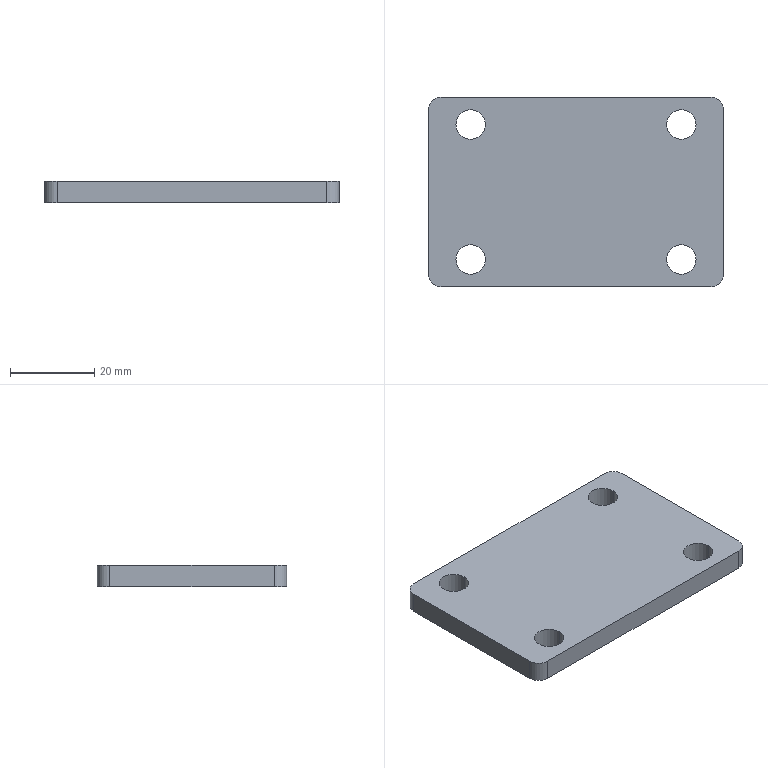Part | SolidWorks | features BaseBody 1 | 1 solid | 18 faces | box 70 x 45 x 5 mm | volume 14942 mm3 | cylinder 12 | plane 6 | commonest cylinder face diameters 7 x8 6 x4
STEP:
#1=CARTESIAN_POINT('',(21.5,-16.,5.));
#2=VERTEX_POINT('',#1);
#3=CARTESIAN_POINT('',(28.5,-16.,5.));
#4=VERTEX_POINT('',#3);
#5=CARTESIAN_POINT('',(25.,-16.,5.));
#6=DIRECTION('',(0.,0.,1.));
#7=DIRECTION('',(1.,0.,0.));
#8=AXIS2_PLACEMENT_3D('',#5,#6,#7);
#9=CIRCLE('',#8,3.5);
#10=EDGE_CURVE('',#2,#4,#9,.T.);
#11=ORIENTED_EDGE('',*,*,#10,.T.);
#12=CARTESIAN_POINT('',(28.5,-16.,0.));
#13=VERTEX_POINT('',#12);
#14=CARTESIAN_POINT('',(28.5,-16.,5.));
#15=DIRECTION('',(0.,0.,-1.));
#16=VECTOR('',#15,1000.);
#17=LINE('',#14,#16);
#18=EDGE_CURVE('',#4,#13,#17,.T.);
#19=ORIENTED_EDGE('',*,*,#18,.T.);
#20=CARTESIAN_POINT('',(21.5,-16.,0.));
#21=VERTEX_POINT('',#20);
#22=CARTESIAN_POINT('',(25.,-16.,0.));
#23=DIRECTION('',(0.,0.,1.));
#24=DIRECTION('',(1.,0.,0.));
#25=AXIS2_PLACEMENT_3D('',#22,#23,#24);
#26=CIRCLE('',#25,3.5);
#27=EDGE_CURVE('',#21,#13,#26,.T.);
#28=ORIENTED_EDGE('',*,*,#27,.F.);
#29=CARTESIAN_POINT('',(21.5,-16.,5.));
#30=DIRECTION('',(0.,0.,-1.));
#31=VECTOR('',#30,1000.);
#32=LINE('',#29,#31);
#33=EDGE_CURVE('',#2,#21,#32,.T.);
#34=ORIENTED_EDGE('',*,*,#33,.F.);
#35=EDGE_LOOP('',(#11,#19,#28,#34));
#36=FACE_OUTER_BOUND('',#35,.T.);
#37=CARTESIAN_POINT('',(25.,-16.,5.));
#38=DIRECTION('',(0.,0.,-1.));
#39=DIRECTION('',(-1.,0.,0.));
#40=AXIS2_PLACEMENT_3D('',#37,#38,#39);
#41=CYLINDRICAL_SURFACE('',#40,3.5);
#42=ADVANCED_FACE('',(#36),#41,.F.);
#43=CARTESIAN_POINT('',(-28.5,-16.,5.));
#44=VERTEX_POINT('',#43);
#45=CARTESIAN_POINT('',(-21.5,-16.,5.));
#46=VERTEX_POINT('',#45);
#47=CARTESIAN_POINT('',(-25.,-16.,5.));
#48=DIRECTION('',(0.,0.,1.));
#49=DIRECTION('',(-1.,0.,0.));
#50=AXIS2_PLACEMENT_3D('',#47,#48,#49);
#51=CIRCLE('',#50,3.5);
#52=EDGE_CURVE('',#44,#46,#51,.T.);
#53=ORIENTED_EDGE('',*,*,#52,.T.);
#54=CARTESIAN_POINT('',(-21.5,-16.,0.));
#55=VERTEX_POINT('',#54);
#56=CARTESIAN_POINT('',(-21.5,-16.,5.));
#57=DIRECTION('',(0.,0.,-1.));
#58=VECTOR('',#57,1000.);
#59=LINE('',#56,#58);
#60=EDGE_CURVE('',#46,#55,#59,.T.);
#61=ORIENTED_EDGE('',*,*,#60,.T.);
#62=CARTESIAN_POINT('',(-28.5,-16.,0.));
#63=VERTEX_POINT('',#62);
#64=CARTESIAN_POINT('',(-25.,-16.,0.));
#65=DIRECTION('',(0.,0.,1.));
#66=DIRECTION('',(-1.,0.,0.));
#67=AXIS2_PLACEMENT_3D('',#64,#65,#66);
#68=CIRCLE('',#67,3.5);
#69=EDGE_CURVE('',#63,#55,#68,.T.);
#70=ORIENTED_EDGE('',*,*,#69,.F.);
#71=CARTESIAN_POINT('',(-28.5,-16.,5.));
#72=DIRECTION('',(0.,0.,-1.));
#73=VECTOR('',#72,1000.);
#74=LINE('',#71,#73);
#75=EDGE_CURVE('',#44,#63,#74,.T.);
#76=ORIENTED_EDGE('',*,*,#75,.F.);
#77=EDGE_LOOP('',(#53,#61,#70,#76));
#78=FACE_OUTER_BOUND('',#77,.T.);
#79=CARTESIAN_POINT('',(-25.,-16.,5.));
#80=DIRECTION('',(0.,0.,-1.));
#81=DIRECTION('',(-1.,0.,0.));
#82=AXIS2_PLACEMENT_3D('',#79,#80,#81);
#83=CYLINDRICAL_SURFACE('',#82,3.5);
#84=ADVANCED_FACE('',(#78),#83,.F.);
#85=CARTESIAN_POINT('',(21.5,16.,5.));
#86=VERTEX_POINT('',#85);
#87=CARTESIAN_POINT('',(28.5,16.,5.));
#88=VERTEX_POINT('',#87);
#89=CARTESIAN_POINT('',(25.,16.,5.));
#90=DIRECTION('',(0.,0.,1.));
#91=DIRECTION('',(-1.,0.,0.));
#92=AXIS2_PLACEMENT_3D('',#89,#90,#91);
#93=CIRCLE('',#92,3.5);
#94=EDGE_CURVE('',#86,#88,#93,.T.);
#95=ORIENTED_EDGE('',*,*,#94,.T.);
#96=CARTESIAN_POINT('',(28.5,16.,0.));
#97=VERTEX_POINT('',#96);
#98=CARTESIAN_POINT('',(28.5,16.,5.));
#99=DIRECTION('',(0.,0.,-1.));
#100=VECTOR('',#99,1000.);
#101=LINE('',#98,#100);
#102=EDGE_CURVE('',#88,#97,#101,.T.);
#103=ORIENTED_EDGE('',*,*,#102,.T.);
#104=CARTESIAN_POINT('',(21.5,16.,0.));
#105=VERTEX_POINT('',#104);
#106=CARTESIAN_POINT('',(25.,16.,0.));
#107=DIRECTION('',(0.,0.,1.));
#108=DIRECTION('',(-1.,0.,0.));
#109=AXIS2_PLACEMENT_3D('',#106,#107,#108);
#110=CIRCLE('',#109,3.5);
#111=EDGE_CURVE('',#105,#97,#110,.T.);
#112=ORIENTED_EDGE('',*,*,#111,.F.);
#113=CARTESIAN_POINT('',(21.5,16.,5.));
#114=DIRECTION('',(0.,0.,-1.));
#115=VECTOR('',#114,1000.);
#116=LINE('',#113,#115);
#117=EDGE_CURVE('',#86,#105,#116,.T.);
#118=ORIENTED_EDGE('',*,*,#117,.F.);
#119=EDGE_LOOP('',(#95,#103,#112,#118));
#120=FACE_OUTER_BOUND('',#119,.T.);
#121=CARTESIAN_POINT('',(25.,16.,5.));
#122=DIRECTION('',(0.,0.,-1.));
#123=DIRECTION('',(-1.,0.,0.));
#124=AXIS2_PLACEMENT_3D('',#121,#122,#123);
#125=CYLINDRICAL_SURFACE('',#124,3.5);
#126=ADVANCED_FACE('',(#120),#125,.F.);
#127=CARTESIAN_POINT('',(-28.5,16.,5.));
#128=VERTEX_POINT('',#127);
#129=CARTESIAN_POINT('',(-21.5,16.,5.));
#130=VERTEX_POINT('',#129);
#131=CARTESIAN_POINT('',(-25.,16.,5.));
#132=DIRECTION('',(0.,0.,1.));
#133=DIRECTION('',(1.,0.,0.));
#134=AXIS2_PLACEMENT_3D('',#131,#132,#133);
#135=CIRCLE('',#134,3.5);
#136=EDGE_CURVE('',#128,#130,#135,.T.);
#137=ORIENTED_EDGE('',*,*,#136,.T.);
#138=CARTESIAN_POINT('',(-21.5,16.,0.));
#139=VERTEX_POINT('',#138);
#140=CARTESIAN_POINT('',(-21.5,16.,5.));
#141=DIRECTION('',(0.,0.,-1.));
#142=VECTOR('',#141,1000.);
#143=LINE('',#140,#142);
#144=EDGE_CURVE('',#130,#139,#143,.T.);
#145=ORIENTED_EDGE('',*,*,#144,.T.);
#146=CARTESIAN_POINT('',(-28.5,16.,0.));
#147=VERTEX_POINT('',#146);
#148=CARTESIAN_POINT('',(-25.,16.,0.));
#149=DIRECTION('',(0.,0.,1.));
#150=DIRECTION('',(1.,0.,0.));
#151=AXIS2_PLACEMENT_3D('',#148,#149,#150);
#152=CIRCLE('',#151,3.5);
#153=EDGE_CURVE('',#147,#139,#152,.T.);
#154=ORIENTED_EDGE('',*,*,#153,.F.);
#155=CARTESIAN_POINT('',(-28.5,16.,5.));
#156=DIRECTION('',(0.,0.,-1.));
#157=VECTOR('',#156,1000.);
#158=LINE('',#155,#157);
#159=EDGE_CURVE('',#128,#147,#158,.T.);
#160=ORIENTED_EDGE('',*,*,#159,.F.);
#161=EDGE_LOOP('',(#137,#145,#154,#160));
#162=FACE_OUTER_BOUND('',#161,.T.);
#163=CARTESIAN_POINT('',(-25.,16.,5.));
#164=DIRECTION('',(0.,0.,-1.));
#165=DIRECTION('',(-1.,0.,0.));
#166=AXIS2_PLACEMENT_3D('',#163,#164,#165);
#167=CYLINDRICAL_SURFACE('',#166,3.5);
#168=ADVANCED_FACE('',(#162),#167,.F.);
#169=CARTESIAN_POINT('',(-35.,19.5,5.));
#170=VERTEX_POINT('',#169);
#171=CARTESIAN_POINT('',(-35.,-19.5,5.));
#172=VERTEX_POINT('',#171);
#173=CARTESIAN_POINT('',(-35.,-22.5,5.));
#174=DIRECTION('',(0.,-1.,0.));
#175=VECTOR('',#174,1000.);
#176=LINE('',#173,#175);
#177=EDGE_CURVE('',#170,#172,#176,.T.);
#178=ORIENTED_EDGE('',*,*,#177,.T.);
#179=CARTESIAN_POINT('',(-32.,-22.5,5.));
#180=VERTEX_POINT('',#179);
#181=CARTESIAN_POINT('',(-32.,-19.5,5.));
#182=DIRECTION('',(0.,0.,1.));
#183=DIRECTION('',(-1.,0.,0.));
#184=AXIS2_PLACEMENT_3D('',#181,#182,#183);
#185=CIRCLE('',#184,3.);
#186=EDGE_CURVE('',#172,#180,#185,.T.);
#187=ORIENTED_EDGE('',*,*,#186,.T.);
#188=CARTESIAN_POINT('',(32.,-22.5,5.));
#189=VERTEX_POINT('',#188);
#190=CARTESIAN_POINT('',(-35.,-22.5,5.));
#191=DIRECTION('',(1.,0.,0.));
#192=VECTOR('',#191,1000.);
#193=LINE('',#190,#192);
#194=EDGE_CURVE('',#180,#189,#193,.T.);
#195=ORIENTED_EDGE('',*,*,#194,.T.);
#196=CARTESIAN_POINT('',(35.,-19.5,5.));
#197=VERTEX_POINT('',#196);
#198=CARTESIAN_POINT('',(32.,-19.5,5.));
#199=DIRECTION('',(0.,0.,1.));
#200=DIRECTION('',(-1.,0.,0.));
#201=AXIS2_PLACEMENT_3D('',#198,#199,#200);
#202=CIRCLE('',#201,3.);
#203=EDGE_CURVE('',#189,#197,#202,.T.);
#204=ORIENTED_EDGE('',*,*,#203,.T.);
#205=CARTESIAN_POINT('',(35.,19.5,5.));
#206=VERTEX_POINT('',#205);
#207=CARTESIAN_POINT('',(35.,-22.5,5.));
#208=DIRECTION('',(0.,1.,0.));
#209=VECTOR('',#208,1000.);
#210=LINE('',#207,#209);
#211=EDGE_CURVE('',#197,#206,#210,.T.);
#212=ORIENTED_EDGE('',*,*,#211,.T.);
#213=CARTESIAN_POINT('',(32.,22.5,5.));
#214=VERTEX_POINT('',#213);
#215=CARTESIAN_POINT('',(32.,19.5,5.));
#216=DIRECTION('',(0.,0.,1.));
#217=DIRECTION('',(-1.,0.,0.));
#218=AXIS2_PLACEMENT_3D('',#215,#216,#217);
#219=CIRCLE('',#218,3.);
#220=EDGE_CURVE('',#206,#214,#219,.T.);
#221=ORIENTED_EDGE('',*,*,#220,.T.);
#222=CARTESIAN_POINT('',(-32.,22.5,5.));
#223=VERTEX_POINT('',#222);
#224=CARTESIAN_POINT('',(-35.,22.5,5.));
#225=DIRECTION('',(-1.,0.,0.));
#226=VECTOR('',#225,1000.);
#227=LINE('',#224,#226);
#228=EDGE_CURVE('',#214,#223,#227,.T.);
#229=ORIENTED_EDGE('',*,*,#228,.T.);
#230=CARTESIAN_POINT('',(-32.,19.5,5.));
#231=DIRECTION('',(0.,0.,1.));
#232=DIRECTION('',(-1.,0.,0.));
#233=AXIS2_PLACEMENT_3D('',#230,#231,#232);
#234=CIRCLE('',#233,3.);
#235=EDGE_CURVE('',#223,#170,#234,.T.);
#236=ORIENTED_EDGE('',*,*,#235,.T.);
#237=EDGE_LOOP('',(#178,#187,#195,#204,#212,#221,#229,#236));
#238=FACE_OUTER_BOUND('',#237,.T.);
#239=ORIENTED_EDGE('',*,*,#136,.F.);
#240=CARTESIAN_POINT('',(-25.,16.,5.));
#241=DIRECTION('',(0.,0.,1.));
#242=DIRECTION('',(1.,0.,0.));
#243=AXIS2_PLACEMENT_3D('',#240,#241,#242);
#244=CIRCLE('',#243,3.5);
#245=EDGE_CURVE('',#130,#128,#244,.T.);
#246=ORIENTED_EDGE('',*,*,#245,.F.);
#247=EDGE_LOOP('',(#239,#246));
#248=FACE_BOUND('',#247,.T.);
#249=ORIENTED_EDGE('',*,*,#94,.F.);
#250=CARTESIAN_POINT('',(25.,16.,5.));
#251=DIRECTION('',(0.,0.,1.));
#252=DIRECTION('',(-1.,0.,0.));
#253=AXIS2_PLACEMENT_3D('',#250,#251,#252);
#254=CIRCLE('',#253,3.5);
#255=EDGE_CURVE('',#88,#86,#254,.T.);
#256=ORIENTED_EDGE('',*,*,#255,.F.);
#257=EDGE_LOOP('',(#249,#256));
#258=FACE_BOUND('',#257,.T.);
#259=ORIENTED_EDGE('',*,*,#52,.F.);
#260=CARTESIAN_POINT('',(-25.,-16.,5.));
#261=DIRECTION('',(0.,0.,1.));
#262=DIRECTION('',(-1.,0.,0.));
#263=AXIS2_PLACEMENT_3D('',#260,#261,#262);
#264=CIRCLE('',#263,3.5);
#265=EDGE_CURVE('',#46,#44,#264,.T.);
#266=ORIENTED_EDGE('',*,*,#265,.F.);
#267=EDGE_LOOP('',(#259,#266));
#268=FACE_BOUND('',#267,.T.);
#269=ORIENTED_EDGE('',*,*,#10,.F.);
#270=CARTESIAN_POINT('',(25.,-16.,5.));
#271=DIRECTION('',(0.,0.,1.));
#272=DIRECTION('',(1.,0.,0.));
#273=AXIS2_PLACEMENT_3D('',#270,#271,#272);
#274=CIRCLE('',#273,3.5);
#275=EDGE_CURVE('',#4,#2,#274,.T.);
#276=ORIENTED_EDGE('',*,*,#275,.F.);
#277=EDGE_LOOP('',(#269,#276));
#278=FACE_BOUND('',#277,.T.);
#279=CARTESIAN_POINT('',(0.,0.,5.));
#280=DIRECTION('',(0.,0.,-1.));
#281=DIRECTION('',(-1.,0.,0.));
#282=AXIS2_PLACEMENT_3D('',#279,#280,#281);
#283=PLANE('',#282);
#284=ADVANCED_FACE('',(#238,#248,#258,#268,#278),#283,.F.);
#285=ORIENTED_EDGE('',*,*,#69,.T.);
#286=CARTESIAN_POINT('',(-25.,-16.,0.));
#287=DIRECTION('',(0.,0.,1.));
#288=DIRECTION('',(-1.,0.,0.));
#289=AXIS2_PLACEMENT_3D('',#286,#287,#288);
#290=CIRCLE('',#289,3.5);
#291=EDGE_CURVE('',#55,#63,#290,.T.);
#292=ORIENTED_EDGE('',*,*,#291,.T.);
#293=EDGE_LOOP('',(#285,#292));
#294=FACE_BOUND('',#293,.T.);
#295=ORIENTED_EDGE('',*,*,#153,.T.);
#296=CARTESIAN_POINT('',(-25.,16.,0.));
#297=DIRECTION('',(0.,0.,1.));
#298=DIRECTION('',(1.,0.,0.));
#299=AXIS2_PLACEMENT_3D('',#296,#297,#298);
#300=CIRCLE('',#299,3.5);
#301=EDGE_CURVE('',#139,#147,#300,.T.);
#302=ORIENTED_EDGE('',*,*,#301,.T.);
#303=EDGE_LOOP('',(#295,#302));
#304=FACE_BOUND('',#303,.T.);
#305=CARTESIAN_POINT('',(-32.,-22.5,0.));
#306=VERTEX_POINT('',#305);
#307=CARTESIAN_POINT('',(32.,-22.5,0.));
#308=VERTEX_POINT('',#307);
#309=CARTESIAN_POINT('',(-35.,-22.5,0.));
#310=DIRECTION('',(1.,0.,0.));
#311=VECTOR('',#310,1000.);
#312=LINE('',#309,#311);
#313=EDGE_CURVE('',#306,#308,#312,.T.);
#314=ORIENTED_EDGE('',*,*,#313,.F.);
#315=CARTESIAN_POINT('',(-35.,-19.5,0.));
#316=VERTEX_POINT('',#315);
#317=CARTESIAN_POINT('',(-32.,-19.5,0.));
#318=DIRECTION('',(0.,0.,-1.));
#319=DIRECTION('',(-1.,0.,0.));
#320=AXIS2_PLACEMENT_3D('',#317,#318,#319);
#321=CIRCLE('',#320,3.);
#322=EDGE_CURVE('',#306,#316,#321,.T.);
#323=ORIENTED_EDGE('',*,*,#322,.T.);
#324=CARTESIAN_POINT('',(-35.,19.5,0.));
#325=VERTEX_POINT('',#324);
#326=CARTESIAN_POINT('',(-35.,-22.5,0.));
#327=DIRECTION('',(0.,-1.,0.));
#328=VECTOR('',#327,1000.);
#329=LINE('',#326,#328);
#330=EDGE_CURVE('',#325,#316,#329,.T.);
#331=ORIENTED_EDGE('',*,*,#330,.F.);
#332=CARTESIAN_POINT('',(-32.,22.5,0.));
#333=VERTEX_POINT('',#332);
#334=CARTESIAN_POINT('',(-32.,19.5,0.));
#335=DIRECTION('',(0.,0.,-1.));
#336=DIRECTION('',(-1.,0.,0.));
#337=AXIS2_PLACEMENT_3D('',#334,#335,#336);
#338=CIRCLE('',#337,3.);
#339=EDGE_CURVE('',#325,#333,#338,.T.);
#340=ORIENTED_EDGE('',*,*,#339,.T.);
#341=CARTESIAN_POINT('',(32.,22.5,0.));
#342=VERTEX_POINT('',#341);
#343=CARTESIAN_POINT('',(-35.,22.5,0.));
#344=DIRECTION('',(-1.,0.,0.));
#345=VECTOR('',#344,1000.);
#346=LINE('',#343,#345);
#347=EDGE_CURVE('',#342,#333,#346,.T.);
#348=ORIENTED_EDGE('',*,*,#347,.F.);
#349=CARTESIAN_POINT('',(35.,19.5,0.));
#350=VERTEX_POINT('',#349);
#351=CARTESIAN_POINT('',(32.,19.5,0.));
#352=DIRECTION('',(0.,0.,-1.));
#353=DIRECTION('',(-1.,0.,0.));
#354=AXIS2_PLACEMENT_3D('',#351,#352,#353);
#355=CIRCLE('',#354,3.);
#356=EDGE_CURVE('',#342,#350,#355,.T.);
#357=ORIENTED_EDGE('',*,*,#356,.T.);
#358=CARTESIAN_POINT('',(35.,-19.5,0.));
#359=VERTEX_POINT('',#358);
#360=CARTESIAN_POINT('',(35.,-22.5,0.));
#361=DIRECTION('',(0.,1.,0.));
#362=VECTOR('',#361,1000.);
#363=LINE('',#360,#362);
#364=EDGE_CURVE('',#359,#350,#363,.T.);
#365=ORIENTED_EDGE('',*,*,#364,.F.);
#366=CARTESIAN_POINT('',(32.,-19.5,0.));
#367=DIRECTION('',(0.,0.,-1.));
#368=DIRECTION('',(-1.,0.,0.));
#369=AXIS2_PLACEMENT_3D('',#366,#367,#368);
#370=CIRCLE('',#369,3.);
#371=EDGE_CURVE('',#359,#308,#370,.T.);
#372=ORIENTED_EDGE('',*,*,#371,.T.);
#373=EDGE_LOOP('',(#314,#323,#331,#340,#348,#357,#365,#372));
#374=FACE_OUTER_BOUND('',#373,.T.);
#375=ORIENTED_EDGE('',*,*,#111,.T.);
#376=CARTESIAN_POINT('',(25.,16.,0.));
#377=DIRECTION('',(0.,0.,1.));
#378=DIRECTION('',(-1.,0.,0.));
#379=AXIS2_PLACEMENT_3D('',#376,#377,#378);
#380=CIRCLE('',#379,3.5);
#381=EDGE_CURVE('',#97,#105,#380,.T.);
#382=ORIENTED_EDGE('',*,*,#381,.T.);
#383=EDGE_LOOP('',(#375,#382));
#384=FACE_BOUND('',#383,.T.);
#385=ORIENTED_EDGE('',*,*,#27,.T.);
#386=CARTESIAN_POINT('',(25.,-16.,0.));
#387=DIRECTION('',(0.,0.,1.));
#388=DIRECTION('',(1.,0.,0.));
#389=AXIS2_PLACEMENT_3D('',#386,#387,#388);
#390=CIRCLE('',#389,3.5);
#391=EDGE_CURVE('',#13,#21,#390,.T.);
#392=ORIENTED_EDGE('',*,*,#391,.T.);
#393=EDGE_LOOP('',(#385,#392));
#394=FACE_BOUND('',#393,.T.);
#395=CARTESIAN_POINT('',(0.,0.,0.));
#396=DIRECTION('',(0.,0.,-1.));
#397=DIRECTION('',(-1.,0.,0.));
#398=AXIS2_PLACEMENT_3D('',#395,#396,#397);
#399=PLANE('',#398);
#400=ADVANCED_FACE('',(#294,#304,#374,#384,#394),#399,.T.);
#401=ORIENTED_EDGE('',*,*,#211,.F.);
#402=CARTESIAN_POINT('',(35.,-19.5,5.));
#403=DIRECTION('',(0.,0.,-1.));
#404=VECTOR('',#403,1000.);
#405=LINE('',#402,#404);
#406=EDGE_CURVE('',#197,#359,#405,.T.);
#407=ORIENTED_EDGE('',*,*,#406,.T.);
#408=ORIENTED_EDGE('',*,*,#364,.T.);
#409=CARTESIAN_POINT('',(35.,19.5,5.));
#410=DIRECTION('',(0.,0.,1.));
#411=VECTOR('',#410,1000.);
#412=LINE('',#409,#411);
#413=EDGE_CURVE('',#350,#206,#412,.T.);
#414=ORIENTED_EDGE('',*,*,#413,.T.);
#415=EDGE_LOOP('',(#401,#407,#408,#414));
#416=FACE_OUTER_BOUND('',#415,.T.);
#417=CARTESIAN_POINT('',(35.,-22.5,5.));
#418=DIRECTION('',(-1.,0.,0.));
#419=DIRECTION('',(0.,0.,1.));
#420=AXIS2_PLACEMENT_3D('',#417,#418,#419);
#421=PLANE('',#420);
#422=ADVANCED_FACE('',(#416),#421,.F.);
#423=ORIENTED_EDGE('',*,*,#228,.F.);
#424=CARTESIAN_POINT('',(32.,22.5,5.));
#425=DIRECTION('',(0.,0.,-1.));
#426=VECTOR('',#425,1000.);
#427=LINE('',#424,#426);
#428=EDGE_CURVE('',#214,#342,#427,.T.);
#429=ORIENTED_EDGE('',*,*,#428,.T.);
#430=ORIENTED_EDGE('',*,*,#347,.T.);
#431=CARTESIAN_POINT('',(-32.,22.5,5.));
#432=DIRECTION('',(0.,0.,1.));
#433=VECTOR('',#432,1000.);
#434=LINE('',#431,#433);
#435=EDGE_CURVE('',#333,#223,#434,.T.);
#436=ORIENTED_EDGE('',*,*,#435,.T.);
#437=EDGE_LOOP('',(#423,#429,#430,#436));
#438=FACE_OUTER_BOUND('',#437,.T.);
#439=CARTESIAN_POINT('',(-35.,22.5,5.));
#440=DIRECTION('',(0.,-1.,0.));
#441=DIRECTION('',(0.,0.,-1.));
#442=AXIS2_PLACEMENT_3D('',#439,#440,#441);
#443=PLANE('',#442);
#444=ADVANCED_FACE('',(#438),#443,.F.);
#445=ORIENTED_EDGE('',*,*,#330,.T.);
#446=CARTESIAN_POINT('',(-35.,-19.5,5.));
#447=DIRECTION('',(0.,0.,1.));
#448=VECTOR('',#447,1000.);
#449=LINE('',#446,#448);
#450=EDGE_CURVE('',#316,#172,#449,.T.);
#451=ORIENTED_EDGE('',*,*,#450,.T.);
#452=ORIENTED_EDGE('',*,*,#177,.F.);
#453=CARTESIAN_POINT('',(-35.,19.5,5.));
#454=DIRECTION('',(0.,0.,-1.));
#455=VECTOR('',#454,1000.);
#456=LINE('',#453,#455);
#457=EDGE_CURVE('',#170,#325,#456,.T.);
#458=ORIENTED_EDGE('',*,*,#457,.T.);
#459=EDGE_LOOP('',(#445,#451,#452,#458));
#460=FACE_OUTER_BOUND('',#459,.T.);
#461=CARTESIAN_POINT('',(-35.,-22.5,5.));
#462=DIRECTION('',(1.,0.,0.));
#463=DIRECTION('',(0.,0.,-1.));
#464=AXIS2_PLACEMENT_3D('',#461,#462,#463);
#465=PLANE('',#464);
#466=ADVANCED_FACE('',(#460),#465,.F.);
#467=ORIENTED_EDGE('',*,*,#194,.F.);
#468=CARTESIAN_POINT('',(-32.,-22.5,5.));
#469=DIRECTION('',(0.,0.,-1.));
#470=VECTOR('',#469,1000.);
#471=LINE('',#468,#470);
#472=EDGE_CURVE('',#180,#306,#471,.T.);
#473=ORIENTED_EDGE('',*,*,#472,.T.);
#474=ORIENTED_EDGE('',*,*,#313,.T.);
#475=CARTESIAN_POINT('',(32.,-22.5,5.));
#476=DIRECTION('',(0.,0.,1.));
#477=VECTOR('',#476,1000.);
#478=LINE('',#475,#477);
#479=EDGE_CURVE('',#308,#189,#478,.T.);
#480=ORIENTED_EDGE('',*,*,#479,.T.);
#481=EDGE_LOOP('',(#467,#473,#474,#480));
#482=FACE_OUTER_BOUND('',#481,.T.);
#483=CARTESIAN_POINT('',(-35.,-22.5,5.));
#484=DIRECTION('',(0.,1.,0.));
#485=DIRECTION('',(0.,0.,1.));
#486=AXIS2_PLACEMENT_3D('',#483,#484,#485);
#487=PLANE('',#486);
#488=ADVANCED_FACE('',(#482),#487,.F.);
#489=ORIENTED_EDGE('',*,*,#144,.F.);
#490=ORIENTED_EDGE('',*,*,#245,.T.);
#491=ORIENTED_EDGE('',*,*,#159,.T.);
#492=ORIENTED_EDGE('',*,*,#301,.F.);
#493=EDGE_LOOP('',(#489,#490,#491,#492));
#494=FACE_OUTER_BOUND('',#493,.T.);
#495=CARTESIAN_POINT('',(-25.,16.,5.));
#496=DIRECTION('',(0.,0.,-1.));
#497=DIRECTION('',(-1.,0.,0.));
#498=AXIS2_PLACEMENT_3D('',#495,#496,#497);
#499=CYLINDRICAL_SURFACE('',#498,3.5);
#500=ADVANCED_FACE('',(#494),#499,.F.);
#501=ORIENTED_EDGE('',*,*,#102,.F.);
#502=ORIENTED_EDGE('',*,*,#255,.T.);
#503=ORIENTED_EDGE('',*,*,#117,.T.);
#504=ORIENTED_EDGE('',*,*,#381,.F.);
#505=EDGE_LOOP('',(#501,#502,#503,#504));
#506=FACE_OUTER_BOUND('',#505,.T.);
#507=CARTESIAN_POINT('',(25.,16.,5.));
#508=DIRECTION('',(0.,0.,-1.));
#509=DIRECTION('',(-1.,0.,0.));
#510=AXIS2_PLACEMENT_3D('',#507,#508,#509);
#511=CYLINDRICAL_SURFACE('',#510,3.5);
#512=ADVANCED_FACE('',(#506),#511,.F.);
#513=ORIENTED_EDGE('',*,*,#60,.F.);
#514=ORIENTED_EDGE('',*,*,#265,.T.);
#515=ORIENTED_EDGE('',*,*,#75,.T.);
#516=ORIENTED_EDGE('',*,*,#291,.F.);
#517=EDGE_LOOP('',(#513,#514,#515,#516));
#518=FACE_OUTER_BOUND('',#517,.T.);
#519=CARTESIAN_POINT('',(-25.,-16.,5.));
#520=DIRECTION('',(0.,0.,-1.));
#521=DIRECTION('',(-1.,0.,0.));
#522=AXIS2_PLACEMENT_3D('',#519,#520,#521);
#523=CYLINDRICAL_SURFACE('',#522,3.5);
#524=ADVANCED_FACE('',(#518),#523,.F.);
#525=ORIENTED_EDGE('',*,*,#18,.F.);
#526=ORIENTED_EDGE('',*,*,#275,.T.);
#527=ORIENTED_EDGE('',*,*,#33,.T.);
#528=ORIENTED_EDGE('',*,*,#391,.F.);
#529=EDGE_LOOP('',(#525,#526,#527,#528));
#530=FACE_OUTER_BOUND('',#529,.T.);
#531=CARTESIAN_POINT('',(25.,-16.,5.));
#532=DIRECTION('',(0.,0.,-1.));
#533=DIRECTION('',(-1.,0.,0.));
#534=AXIS2_PLACEMENT_3D('',#531,#532,#533);
#535=CYLINDRICAL_SURFACE('',#534,3.5);
#536=ADVANCED_FACE('',(#530),#535,.F.);
#537=ORIENTED_EDGE('',*,*,#186,.F.);
#538=ORIENTED_EDGE('',*,*,#450,.F.);
#539=ORIENTED_EDGE('',*,*,#322,.F.);
#540=ORIENTED_EDGE('',*,*,#472,.F.);
#541=EDGE_LOOP('',(#537,#538,#539,#540));
#542=FACE_OUTER_BOUND('',#541,.T.);
#543=CARTESIAN_POINT('',(-32.,-19.5,5.));
#544=DIRECTION('',(0.,0.,-1.));
#545=DIRECTION('',(-1.,0.,0.));
#546=AXIS2_PLACEMENT_3D('',#543,#544,#545);
#547=CYLINDRICAL_SURFACE('',#546,3.);
#548=ADVANCED_FACE('',(#542),#547,.T.);
#549=ORIENTED_EDGE('',*,*,#203,.F.);
#550=ORIENTED_EDGE('',*,*,#479,.F.);
#551=ORIENTED_EDGE('',*,*,#371,.F.);
#552=ORIENTED_EDGE('',*,*,#406,.F.);
#553=EDGE_LOOP('',(#549,#550,#551,#552));
#554=FACE_OUTER_BOUND('',#553,.T.);
#555=CARTESIAN_POINT('',(32.,-19.5,5.));
#556=DIRECTION('',(0.,0.,-1.));
#557=DIRECTION('',(-1.,0.,0.));
#558=AXIS2_PLACEMENT_3D('',#555,#556,#557);
#559=CYLINDRICAL_SURFACE('',#558,3.);
#560=ADVANCED_FACE('',(#554),#559,.T.);
#561=ORIENTED_EDGE('',*,*,#220,.F.);
#562=ORIENTED_EDGE('',*,*,#413,.F.);
#563=ORIENTED_EDGE('',*,*,#356,.F.);
#564=ORIENTED_EDGE('',*,*,#428,.F.);
#565=EDGE_LOOP('',(#561,#562,#563,#564));
#566=FACE_OUTER_BOUND('',#565,.T.);
#567=CARTESIAN_POINT('',(32.,19.5,5.));
#568=DIRECTION('',(0.,0.,-1.));
#569=DIRECTION('',(-1.,0.,0.));
#570=AXIS2_PLACEMENT_3D('',#567,#568,#569);
#571=CYLINDRICAL_SURFACE('',#570,3.);
#572=ADVANCED_FACE('',(#566),#571,.T.);
#573=ORIENTED_EDGE('',*,*,#235,.F.);
#574=ORIENTED_EDGE('',*,*,#435,.F.);
#575=ORIENTED_EDGE('',*,*,#339,.F.);
#576=ORIENTED_EDGE('',*,*,#457,.F.);
#577=EDGE_LOOP('',(#573,#574,#575,#576));
#578=FACE_OUTER_BOUND('',#577,.T.);
#579=CARTESIAN_POINT('',(-32.,19.5,5.));
#580=DIRECTION('',(0.,0.,-1.));
#581=DIRECTION('',(-1.,0.,0.));
#582=AXIS2_PLACEMENT_3D('',#579,#580,#581);
#583=CYLINDRICAL_SURFACE('',#582,3.);
#584=ADVANCED_FACE('',(#578),#583,.T.);
#585=CLOSED_SHELL('',(#42,#84,#126,#168,#284,#400,#422,#444,#466,#488,#500,#512,#524,#536,#548,#560,#572,#584));
#586=MANIFOLD_SOLID_BREP('',#585);
#587=CARTESIAN_POINT('',(0.,0.,0.));
#588=DIRECTION('',(0.,0.,1.));
#589=DIRECTION('',(1.,0.,0.));
#590=AXIS2_PLACEMENT_3D('',#587,#588,#589);
#591=(LENGTH_UNIT()NAMED_UNIT(*)SI_UNIT(.MILLI.,.METRE.));
#592=UNCERTAINTY_MEASURE_WITH_UNIT(LENGTH_MEASURE(0.00001),#591,'','');
#593=(NAMED_UNIT(*)PLANE_ANGLE_UNIT()SI_UNIT($,.RADIAN.));
#594=(NAMED_UNIT(*)SI_UNIT($,.STERADIAN.)SOLID_ANGLE_UNIT());
#595=(GEOMETRIC_REPRESENTATION_CONTEXT(3)GLOBAL_UNCERTAINTY_ASSIGNED_CONTEXT((#592))GLOBAL_UNIT_ASSIGNED_CONTEXT((#591,#593,#594))REPRESENTATION_CONTEXT('',''));
#596=ADVANCED_BREP_SHAPE_REPRESENTATION('',(#586,#590),#595);